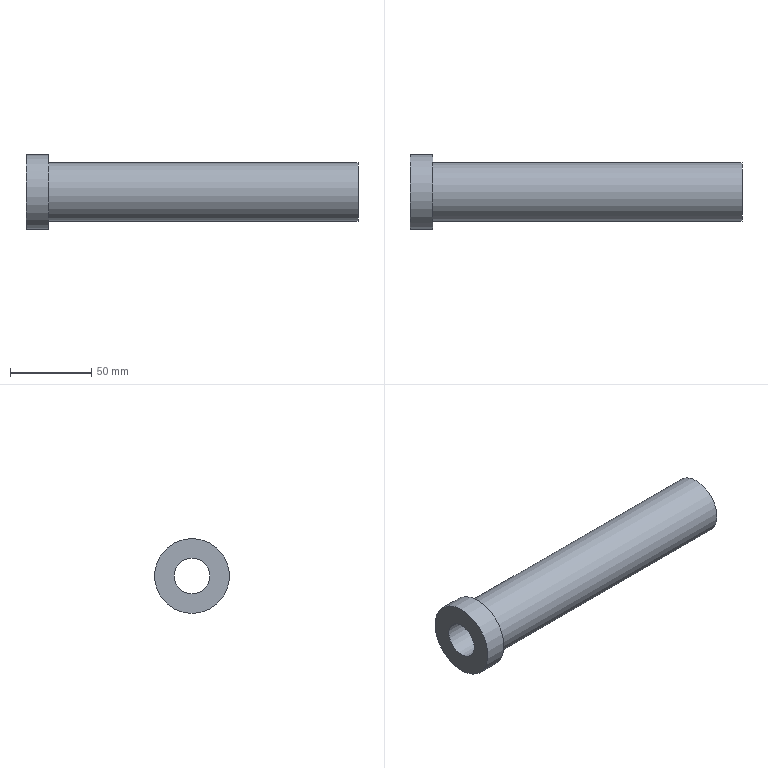Part | STEP file | solid 149 | 1 solid | 6 faces | box 204 x 46 x 46 mm | volume 139116 mm3 | plane 3 | cylinder 3 | commonest cylinder face diameters 22 x1 36 x1 46 x1